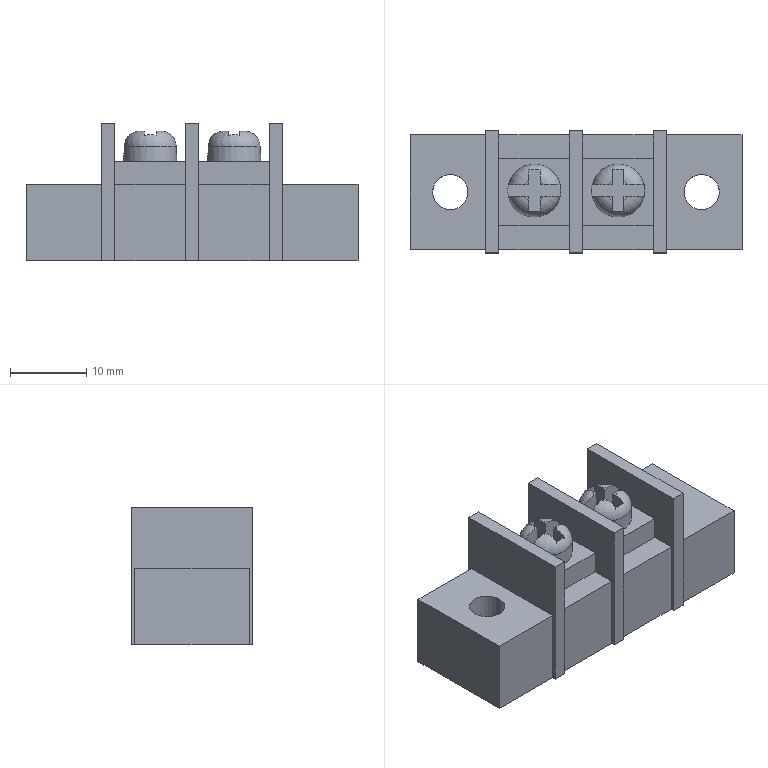Part | NX | features BREP 1 | 1 solid | 76 faces | box 43.584 x 16 x 18 mm | volume 7630 mm3 | plane 68 | cylinder 4 | torus 4 | commonest cylinder face diameters 4.637 x2 6.956 x2